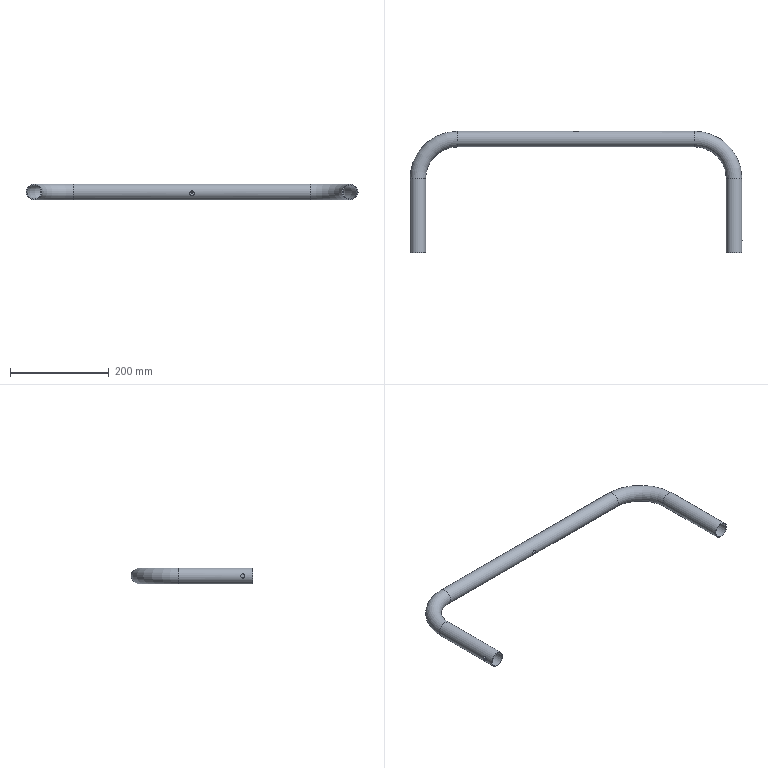Part | STEP file | 6101301 | 1 solid | 16 faces | box 671.8 x 245.9 x 31.8 mm | volume 146844 mm3 | cylinder 10 | torus 4 | plane 2 | commonest cylinder face diameters 28.8 x3 31.8 x3 8.5 x2 10 x2